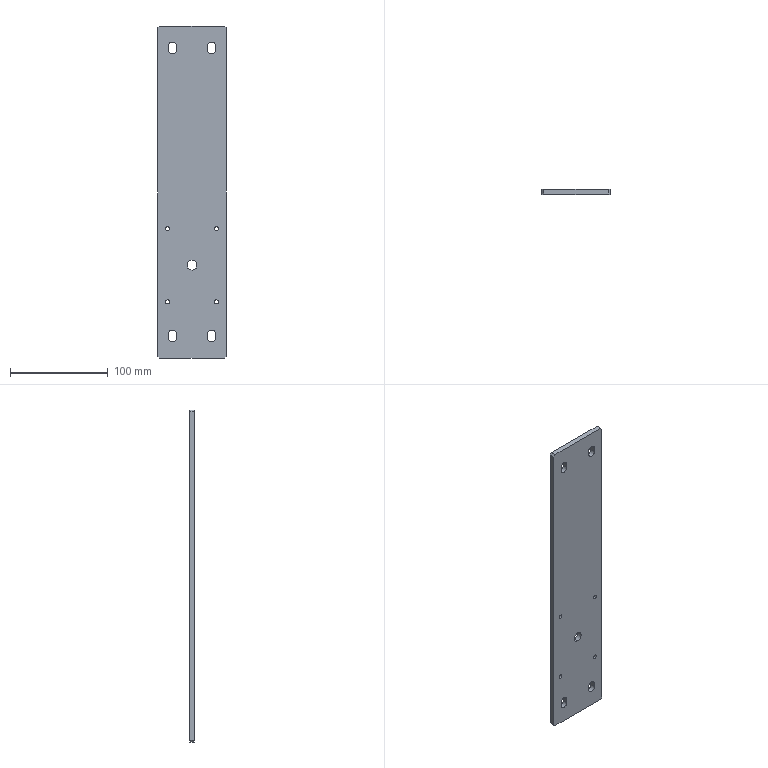Part | SolidWorks | features HoleWzd 2, Chamfer 1, Extrusion 1, ICE 1 | 1 solid | 40 faces | box 70 x 5 x 340 mm | volume 116578 mm3 | cylinder 22 | plane 18 | commonest cylinder face diameters 8.2 x12 4.2 x8 10 x2
STEP:
#1=CARTESIAN_POINT('',(-25.,0.,-110.4));
#2=VERTEX_POINT('',#1);
#3=CARTESIAN_POINT('',(-25.,0.,-114.6));
#4=VERTEX_POINT('',#3);
#5=CARTESIAN_POINT('',(-25.,0.,-112.5));
#6=DIRECTION('',(0.,-1.,0.));
#7=DIRECTION('',(0.,0.,-1.));
#8=AXIS2_PLACEMENT_3D('',#5,#6,#7);
#9=CIRCLE('',#8,2.1);
#10=EDGE_CURVE('',#2,#4,#9,.T.);
#11=ORIENTED_EDGE('',*,*,#10,.T.);
#12=CARTESIAN_POINT('',(-25.,5.,-114.6));
#13=VERTEX_POINT('',#12);
#14=CARTESIAN_POINT('',(-25.,5.,-114.6));
#15=DIRECTION('',(0.,1.,0.));
#16=VECTOR('',#15,1000.);
#17=LINE('',#14,#16);
#18=EDGE_CURVE('',#4,#13,#17,.T.);
#19=ORIENTED_EDGE('',*,*,#18,.T.);
#20=CARTESIAN_POINT('',(-25.,5.,-110.4));
#21=VERTEX_POINT('',#20);
#22=CARTESIAN_POINT('',(-25.,5.,-112.5));
#23=DIRECTION('',(0.,1.,0.));
#24=DIRECTION('',(0.,0.,1.));
#25=AXIS2_PLACEMENT_3D('',#22,#23,#24);
#26=CIRCLE('',#25,2.1);
#27=EDGE_CURVE('',#13,#21,#26,.T.);
#28=ORIENTED_EDGE('',*,*,#27,.T.);
#29=CARTESIAN_POINT('',(-25.,5.,-110.4));
#30=DIRECTION('',(0.,1.,0.));
#31=VECTOR('',#30,1000.);
#32=LINE('',#29,#31);
#33=EDGE_CURVE('',#2,#21,#32,.T.);
#34=ORIENTED_EDGE('',*,*,#33,.F.);
#35=EDGE_LOOP('',(#11,#19,#28,#34));
#36=FACE_OUTER_BOUND('',#35,.T.);
#37=CARTESIAN_POINT('',(-25.,5.,-112.5));
#38=DIRECTION('',(0.,1.,0.));
#39=DIRECTION('',(0.,0.,1.));
#40=AXIS2_PLACEMENT_3D('',#37,#38,#39);
#41=CYLINDRICAL_SURFACE('',#40,2.1);
#42=ADVANCED_FACE('',(#36),#41,.F.);
#43=CARTESIAN_POINT('',(25.,0.,-35.4));
#44=VERTEX_POINT('',#43);
#45=CARTESIAN_POINT('',(25.,0.,-39.6));
#46=VERTEX_POINT('',#45);
#47=CARTESIAN_POINT('',(25.,0.,-37.5));
#48=DIRECTION('',(0.,-1.,0.));
#49=DIRECTION('',(0.,0.,-1.));
#50=AXIS2_PLACEMENT_3D('',#47,#48,#49);
#51=CIRCLE('',#50,2.1);
#52=EDGE_CURVE('',#44,#46,#51,.T.);
#53=ORIENTED_EDGE('',*,*,#52,.T.);
#54=CARTESIAN_POINT('',(25.,5.,-39.6));
#55=VERTEX_POINT('',#54);
#56=CARTESIAN_POINT('',(25.,5.,-39.6));
#57=DIRECTION('',(0.,1.,0.));
#58=VECTOR('',#57,1000.);
#59=LINE('',#56,#58);
#60=EDGE_CURVE('',#46,#55,#59,.T.);
#61=ORIENTED_EDGE('',*,*,#60,.T.);
#62=CARTESIAN_POINT('',(25.,5.,-35.4));
#63=VERTEX_POINT('',#62);
#64=CARTESIAN_POINT('',(25.,5.,-37.5));
#65=DIRECTION('',(0.,1.,0.));
#66=DIRECTION('',(0.,0.,1.));
#67=AXIS2_PLACEMENT_3D('',#64,#65,#66);
#68=CIRCLE('',#67,2.1);
#69=EDGE_CURVE('',#55,#63,#68,.T.);
#70=ORIENTED_EDGE('',*,*,#69,.T.);
#71=CARTESIAN_POINT('',(25.,5.,-35.4));
#72=DIRECTION('',(0.,1.,0.));
#73=VECTOR('',#72,1000.);
#74=LINE('',#71,#73);
#75=EDGE_CURVE('',#44,#63,#74,.T.);
#76=ORIENTED_EDGE('',*,*,#75,.F.);
#77=EDGE_LOOP('',(#53,#61,#70,#76));
#78=FACE_OUTER_BOUND('',#77,.T.);
#79=CARTESIAN_POINT('',(25.,5.,-37.5));
#80=DIRECTION('',(0.,1.,0.));
#81=DIRECTION('',(0.,0.,1.));
#82=AXIS2_PLACEMENT_3D('',#79,#80,#81);
#83=CYLINDRICAL_SURFACE('',#82,2.1);
#84=ADVANCED_FACE('',(#78),#83,.F.);
#85=CARTESIAN_POINT('',(-25.,0.,-35.4));
#86=VERTEX_POINT('',#85);
#87=CARTESIAN_POINT('',(-25.,0.,-39.6));
#88=VERTEX_POINT('',#87);
#89=CARTESIAN_POINT('',(-25.,0.,-37.5));
#90=DIRECTION('',(0.,-1.,0.));
#91=DIRECTION('',(0.,0.,-1.));
#92=AXIS2_PLACEMENT_3D('',#89,#90,#91);
#93=CIRCLE('',#92,2.1);
#94=EDGE_CURVE('',#86,#88,#93,.T.);
#95=ORIENTED_EDGE('',*,*,#94,.T.);
#96=CARTESIAN_POINT('',(-25.,5.,-39.6));
#97=VERTEX_POINT('',#96);
#98=CARTESIAN_POINT('',(-25.,5.,-39.6));
#99=DIRECTION('',(0.,1.,0.));
#100=VECTOR('',#99,1000.);
#101=LINE('',#98,#100);
#102=EDGE_CURVE('',#88,#97,#101,.T.);
#103=ORIENTED_EDGE('',*,*,#102,.T.);
#104=CARTESIAN_POINT('',(-25.,5.,-35.4));
#105=VERTEX_POINT('',#104);
#106=CARTESIAN_POINT('',(-25.,5.,-37.5));
#107=DIRECTION('',(0.,1.,0.));
#108=DIRECTION('',(0.,0.,1.));
#109=AXIS2_PLACEMENT_3D('',#106,#107,#108);
#110=CIRCLE('',#109,2.1);
#111=EDGE_CURVE('',#97,#105,#110,.T.);
#112=ORIENTED_EDGE('',*,*,#111,.T.);
#113=CARTESIAN_POINT('',(-25.,5.,-35.4));
#114=DIRECTION('',(0.,1.,0.));
#115=VECTOR('',#114,1000.);
#116=LINE('',#113,#115);
#117=EDGE_CURVE('',#86,#105,#116,.T.);
#118=ORIENTED_EDGE('',*,*,#117,.F.);
#119=EDGE_LOOP('',(#95,#103,#112,#118));
#120=FACE_OUTER_BOUND('',#119,.T.);
#121=CARTESIAN_POINT('',(-25.,5.,-37.5));
#122=DIRECTION('',(0.,1.,0.));
#123=DIRECTION('',(0.,0.,1.));
#124=AXIS2_PLACEMENT_3D('',#121,#122,#123);
#125=CYLINDRICAL_SURFACE('',#124,2.1);
#126=ADVANCED_FACE('',(#120),#125,.F.);
#127=CARTESIAN_POINT('',(25.,0.,-110.4));
#128=VERTEX_POINT('',#127);
#129=CARTESIAN_POINT('',(25.,0.,-114.6));
#130=VERTEX_POINT('',#129);
#131=CARTESIAN_POINT('',(25.,0.,-112.5));
#132=DIRECTION('',(0.,-1.,0.));
#133=DIRECTION('',(0.,0.,-1.));
#134=AXIS2_PLACEMENT_3D('',#131,#132,#133);
#135=CIRCLE('',#134,2.1);
#136=EDGE_CURVE('',#128,#130,#135,.T.);
#137=ORIENTED_EDGE('',*,*,#136,.T.);
#138=CARTESIAN_POINT('',(25.,5.,-114.6));
#139=VERTEX_POINT('',#138);
#140=CARTESIAN_POINT('',(25.,5.,-114.6));
#141=DIRECTION('',(0.,1.,0.));
#142=VECTOR('',#141,1000.);
#143=LINE('',#140,#142);
#144=EDGE_CURVE('',#130,#139,#143,.T.);
#145=ORIENTED_EDGE('',*,*,#144,.T.);
#146=CARTESIAN_POINT('',(25.,5.,-110.4));
#147=VERTEX_POINT('',#146);
#148=CARTESIAN_POINT('',(25.,5.,-112.5));
#149=DIRECTION('',(0.,1.,0.));
#150=DIRECTION('',(0.,0.,1.));
#151=AXIS2_PLACEMENT_3D('',#148,#149,#150);
#152=CIRCLE('',#151,2.1);
#153=EDGE_CURVE('',#139,#147,#152,.T.);
#154=ORIENTED_EDGE('',*,*,#153,.T.);
#155=CARTESIAN_POINT('',(25.,5.,-110.4));
#156=DIRECTION('',(0.,1.,0.));
#157=VECTOR('',#156,1000.);
#158=LINE('',#155,#157);
#159=EDGE_CURVE('',#128,#147,#158,.T.);
#160=ORIENTED_EDGE('',*,*,#159,.F.);
#161=EDGE_LOOP('',(#137,#145,#154,#160));
#162=FACE_OUTER_BOUND('',#161,.T.);
#163=CARTESIAN_POINT('',(25.,5.,-112.5));
#164=DIRECTION('',(0.,1.,0.));
#165=DIRECTION('',(0.,0.,1.));
#166=AXIS2_PLACEMENT_3D('',#163,#164,#165);
#167=CYLINDRICAL_SURFACE('',#166,2.1);
#168=ADVANCED_FACE('',(#162),#167,.F.);
#169=CARTESIAN_POINT('',(0.,0.,-80.));
#170=VERTEX_POINT('',#169);
#171=CARTESIAN_POINT('',(0.,0.,-70.));
#172=VERTEX_POINT('',#171);
#173=CARTESIAN_POINT('',(0.,0.,-75.));
#174=DIRECTION('',(0.,1.,0.));
#175=DIRECTION('',(0.,0.,1.));
#176=AXIS2_PLACEMENT_3D('',#173,#174,#175);
#177=CIRCLE('',#176,5.);
#178=EDGE_CURVE('',#170,#172,#177,.T.);
#179=ORIENTED_EDGE('',*,*,#178,.F.);
#180=CARTESIAN_POINT('',(0.,5.,-80.));
#181=VERTEX_POINT('',#180);
#182=CARTESIAN_POINT('',(0.,0.,-80.));
#183=DIRECTION('',(0.,1.,0.));
#184=VECTOR('',#183,1000.);
#185=LINE('',#182,#184);
#186=EDGE_CURVE('',#170,#181,#185,.T.);
#187=ORIENTED_EDGE('',*,*,#186,.T.);
#188=CARTESIAN_POINT('',(0.,5.,-70.));
#189=VERTEX_POINT('',#188);
#190=CARTESIAN_POINT('',(0.,5.,-75.));
#191=DIRECTION('',(0.,1.,0.));
#192=DIRECTION('',(0.,0.,1.));
#193=AXIS2_PLACEMENT_3D('',#190,#191,#192);
#194=CIRCLE('',#193,5.);
#195=EDGE_CURVE('',#181,#189,#194,.T.);
#196=ORIENTED_EDGE('',*,*,#195,.T.);
#197=CARTESIAN_POINT('',(0.,0.,-70.));
#198=DIRECTION('',(0.,1.,0.));
#199=VECTOR('',#198,1000.);
#200=LINE('',#197,#199);
#201=EDGE_CURVE('',#172,#189,#200,.T.);
#202=ORIENTED_EDGE('',*,*,#201,.F.);
#203=EDGE_LOOP('',(#179,#187,#196,#202));
#204=FACE_OUTER_BOUND('',#203,.T.);
#205=CARTESIAN_POINT('',(0.,0.,-75.));
#206=DIRECTION('',(0.,1.,0.));
#207=DIRECTION('',(0.,0.,1.));
#208=AXIS2_PLACEMENT_3D('',#205,#206,#207);
#209=CYLINDRICAL_SURFACE('',#208,5.);
#210=ADVANCED_FACE('',(#204),#209,.F.);
#211=CARTESIAN_POINT('',(24.1,0.,-145.5));
#212=VERTEX_POINT('',#211);
#213=CARTESIAN_POINT('',(20.,0.,-141.4));
#214=VERTEX_POINT('',#213);
#215=CARTESIAN_POINT('',(20.,0.,-145.5));
#216=DIRECTION('',(0.,-1.,0.));
#217=DIRECTION('',(0.,0.,-1.));
#218=AXIS2_PLACEMENT_3D('',#215,#216,#217);
#219=CIRCLE('',#218,4.1);
#220=EDGE_CURVE('',#212,#214,#219,.T.);
#221=ORIENTED_EDGE('',*,*,#220,.T.);
#222=CARTESIAN_POINT('',(20.,5.,-141.4));
#223=VERTEX_POINT('',#222);
#224=CARTESIAN_POINT('',(20.,5.,-141.4));
#225=DIRECTION('',(0.,1.,0.));
#226=VECTOR('',#225,1000.);
#227=LINE('',#224,#226);
#228=EDGE_CURVE('',#214,#223,#227,.T.);
#229=ORIENTED_EDGE('',*,*,#228,.T.);
#230=CARTESIAN_POINT('',(24.1,5.,-145.5));
#231=VERTEX_POINT('',#230);
#232=CARTESIAN_POINT('',(20.,5.,-145.5));
#233=DIRECTION('',(0.,1.,0.));
#234=DIRECTION('',(0.,0.,1.));
#235=AXIS2_PLACEMENT_3D('',#232,#233,#234);
#236=CIRCLE('',#235,4.1);
#237=EDGE_CURVE('',#223,#231,#236,.T.);
#238=ORIENTED_EDGE('',*,*,#237,.T.);
#239=CARTESIAN_POINT('',(24.1,-10.,-145.5));
#240=DIRECTION('',(0.,-1.,0.));
#241=VECTOR('',#240,1000.);
#242=LINE('',#239,#241);
#243=EDGE_CURVE('',#231,#212,#242,.T.);
#244=ORIENTED_EDGE('',*,*,#243,.T.);
#245=EDGE_LOOP('',(#221,#229,#238,#244));
#246=FACE_OUTER_BOUND('',#245,.T.);
#247=CARTESIAN_POINT('',(20.,5.,-145.5));
#248=DIRECTION('',(0.,1.,0.));
#249=DIRECTION('',(0.,0.,1.));
#250=AXIS2_PLACEMENT_3D('',#247,#248,#249);
#251=CYLINDRICAL_SURFACE('',#250,4.1);
#252=ADVANCED_FACE('',(#246),#251,.F.);
#253=CARTESIAN_POINT('',(-15.9,0.,-145.5));
#254=VERTEX_POINT('',#253);
#255=CARTESIAN_POINT('',(-20.,0.,-141.4));
#256=VERTEX_POINT('',#255);
#257=CARTESIAN_POINT('',(-20.,0.,-145.5));
#258=DIRECTION('',(0.,-1.,0.));
#259=DIRECTION('',(0.,0.,-1.));
#260=AXIS2_PLACEMENT_3D('',#257,#258,#259);
#261=CIRCLE('',#260,4.1);
#262=EDGE_CURVE('',#254,#256,#261,.T.);
#263=ORIENTED_EDGE('',*,*,#262,.T.);
#264=CARTESIAN_POINT('',(-20.,5.,-141.4));
#265=VERTEX_POINT('',#264);
#266=CARTESIAN_POINT('',(-20.,5.,-141.4));
#267=DIRECTION('',(0.,1.,0.));
#268=VECTOR('',#267,1000.);
#269=LINE('',#266,#268);
#270=EDGE_CURVE('',#256,#265,#269,.T.);
#271=ORIENTED_EDGE('',*,*,#270,.T.);
#272=CARTESIAN_POINT('',(-15.9,5.,-145.5));
#273=VERTEX_POINT('',#272);
#274=CARTESIAN_POINT('',(-20.,5.,-145.5));
#275=DIRECTION('',(0.,1.,0.));
#276=DIRECTION('',(0.,0.,1.));
#277=AXIS2_PLACEMENT_3D('',#274,#275,#276);
#278=CIRCLE('',#277,4.1);
#279=EDGE_CURVE('',#265,#273,#278,.T.);
#280=ORIENTED_EDGE('',*,*,#279,.T.);
#281=CARTESIAN_POINT('',(-15.9,-10.,-145.5));
#282=DIRECTION('',(0.,-1.,0.));
#283=VECTOR('',#282,1000.);
#284=LINE('',#281,#283);
#285=EDGE_CURVE('',#273,#254,#284,.T.);
#286=ORIENTED_EDGE('',*,*,#285,.T.);
#287=EDGE_LOOP('',(#263,#271,#280,#286));
#288=FACE_OUTER_BOUND('',#287,.T.);
#289=CARTESIAN_POINT('',(-20.,5.,-145.5));
#290=DIRECTION('',(0.,1.,0.));
#291=DIRECTION('',(0.,0.,1.));
#292=AXIS2_PLACEMENT_3D('',#289,#290,#291);
#293=CYLINDRICAL_SURFACE('',#292,4.1);
#294=ADVANCED_FACE('',(#288),#293,.F.);
#295=CARTESIAN_POINT('',(-15.9,0.,149.5));
#296=VERTEX_POINT('',#295);
#297=CARTESIAN_POINT('',(-20.,0.,153.6));
#298=VERTEX_POINT('',#297);
#299=CARTESIAN_POINT('',(-20.,0.,149.5));
#300=DIRECTION('',(0.,-1.,0.));
#301=DIRECTION('',(0.,0.,-1.));
#302=AXIS2_PLACEMENT_3D('',#299,#300,#301);
#303=CIRCLE('',#302,4.1);
#304=EDGE_CURVE('',#296,#298,#303,.T.);
#305=ORIENTED_EDGE('',*,*,#304,.T.);
#306=CARTESIAN_POINT('',(-20.,5.,153.6));
#307=VERTEX_POINT('',#306);
#308=CARTESIAN_POINT('',(-20.,5.,153.6));
#309=DIRECTION('',(0.,1.,0.));
#310=VECTOR('',#309,1000.);
#311=LINE('',#308,#310);
#312=EDGE_CURVE('',#298,#307,#311,.T.);
#313=ORIENTED_EDGE('',*,*,#312,.T.);
#314=CARTESIAN_POINT('',(-15.9,5.,149.5));
#315=VERTEX_POINT('',#314);
#316=CARTESIAN_POINT('',(-20.,5.,149.5));
#317=DIRECTION('',(0.,1.,0.));
#318=DIRECTION('',(0.,0.,1.));
#319=AXIS2_PLACEMENT_3D('',#316,#317,#318);
#320=CIRCLE('',#319,4.1);
#321=EDGE_CURVE('',#307,#315,#320,.T.);
#322=ORIENTED_EDGE('',*,*,#321,.T.);
#323=CARTESIAN_POINT('',(-15.9,-10.,149.5));
#324=DIRECTION('',(0.,-1.,0.));
#325=VECTOR('',#324,1000.);
#326=LINE('',#323,#325);
#327=EDGE_CURVE('',#315,#296,#326,.T.);
#328=ORIENTED_EDGE('',*,*,#327,.T.);
#329=EDGE_LOOP('',(#305,#313,#322,#328));
#330=FACE_OUTER_BOUND('',#329,.T.);
#331=CARTESIAN_POINT('',(-20.,5.,149.5));
#332=DIRECTION('',(0.,1.,0.));
#333=DIRECTION('',(0.,0.,1.));
#334=AXIS2_PLACEMENT_3D('',#331,#332,#333);
#335=CYLINDRICAL_SURFACE('',#334,4.1);
#336=ADVANCED_FACE('',(#330),#335,.F.);
#337=CARTESIAN_POINT('',(24.1,0.,149.5));
#338=VERTEX_POINT('',#337);
#339=CARTESIAN_POINT('',(20.,0.,153.6));
#340=VERTEX_POINT('',#339);
#341=CARTESIAN_POINT('',(20.,0.,149.5));
#342=DIRECTION('',(0.,-1.,0.));
#343=DIRECTION('',(0.,0.,-1.));
#344=AXIS2_PLACEMENT_3D('',#341,#342,#343);
#345=CIRCLE('',#344,4.1);
#346=EDGE_CURVE('',#338,#340,#345,.T.);
#347=ORIENTED_EDGE('',*,*,#346,.T.);
#348=CARTESIAN_POINT('',(20.,5.,153.6));
#349=VERTEX_POINT('',#348);
#350=CARTESIAN_POINT('',(20.,5.,153.6));
#351=DIRECTION('',(0.,1.,0.));
#352=VECTOR('',#351,1000.);
#353=LINE('',#350,#352);
#354=EDGE_CURVE('',#340,#349,#353,.T.);
#355=ORIENTED_EDGE('',*,*,#354,.T.);
#356=CARTESIAN_POINT('',(24.1,5.,149.5));
#357=VERTEX_POINT('',#356);
#358=CARTESIAN_POINT('',(20.,5.,149.5));
#359=DIRECTION('',(0.,1.,0.));
#360=DIRECTION('',(0.,0.,1.));
#361=AXIS2_PLACEMENT_3D('',#358,#359,#360);
#362=CIRCLE('',#361,4.1);
#363=EDGE_CURVE('',#349,#357,#362,.T.);
#364=ORIENTED_EDGE('',*,*,#363,.T.);
#365=CARTESIAN_POINT('',(24.1,-10.,149.5));
#366=DIRECTION('',(0.,-1.,0.));
#367=VECTOR('',#366,1000.);
#368=LINE('',#365,#367);
#369=EDGE_CURVE('',#357,#338,#368,.T.);
#370=ORIENTED_EDGE('',*,*,#369,.T.);
#371=EDGE_LOOP('',(#347,#355,#364,#370));
#372=FACE_OUTER_BOUND('',#371,.T.);
#373=CARTESIAN_POINT('',(20.,5.,149.5));
#374=DIRECTION('',(0.,1.,0.));
#375=DIRECTION('',(0.,0.,1.));
#376=AXIS2_PLACEMENT_3D('',#373,#374,#375);
#377=CYLINDRICAL_SURFACE('',#376,4.1);
#378=ADVANCED_FACE('',(#372),#377,.F.);
#379=CARTESIAN_POINT('',(35.,0.,168.));
#380=VERTEX_POINT('',#379);
#381=CARTESIAN_POINT('',(35.,0.,-168.));
#382=VERTEX_POINT('',#381);
#383=CARTESIAN_POINT('',(35.,0.,170.));
#384=DIRECTION('',(0.,0.,-1.));
#385=VECTOR('',#384,1000.);
#386=LINE('',#383,#385);
#387=EDGE_CURVE('',#380,#382,#386,.T.);
#388=ORIENTED_EDGE('',*,*,#387,.T.);
#389=CARTESIAN_POINT('',(35.,5.,-168.));
#390=VERTEX_POINT('',#389);
#391=CARTESIAN_POINT('',(35.,5.,-168.));
#392=DIRECTION('',(0.,1.,0.));
#393=VECTOR('',#392,1000.);
#394=LINE('',#391,#393);
#395=EDGE_CURVE('',#382,#390,#394,.T.);
#396=ORIENTED_EDGE('',*,*,#395,.T.);
#397=CARTESIAN_POINT('',(35.,5.,168.));
#398=VERTEX_POINT('',#397);
#399=CARTESIAN_POINT('',(35.,5.,170.));
#400=DIRECTION('',(0.,0.,-1.));
#401=VECTOR('',#400,1000.);
#402=LINE('',#399,#401);
#403=EDGE_CURVE('',#398,#390,#402,.T.);
#404=ORIENTED_EDGE('',*,*,#403,.F.);
#405=CARTESIAN_POINT('',(35.,5.,168.));
#406=DIRECTION('',(0.,-1.,0.));
#407=VECTOR('',#406,1000.);
#408=LINE('',#405,#407);
#409=EDGE_CURVE('',#398,#380,#408,.T.);
#410=ORIENTED_EDGE('',*,*,#409,.T.);
#411=EDGE_LOOP('',(#388,#396,#404,#410));
#412=FACE_OUTER_BOUND('',#411,.T.);
#413=CARTESIAN_POINT('',(35.,5.,170.));
#414=DIRECTION('',(-1.,0.,0.));
#415=DIRECTION('',(0.,0.,1.));
#416=AXIS2_PLACEMENT_3D('',#413,#414,#415);
#417=PLANE('',#416);
#418=ADVANCED_FACE('',(#412),#417,.F.);
#419=CARTESIAN_POINT('',(33.,0.,-170.));
#420=VERTEX_POINT('',#419);
#421=CARTESIAN_POINT('',(-33.,0.,-170.));
#422=VERTEX_POINT('',#421);
#423=CARTESIAN_POINT('',(-35.,0.,-170.));
#424=DIRECTION('',(-1.,0.,0.));
#425=VECTOR('',#424,1000.);
#426=LINE('',#423,#425);
#427=EDGE_CURVE('',#420,#422,#426,.T.);
#428=ORIENTED_EDGE('',*,*,#427,.T.);
#429=CARTESIAN_POINT('',(-33.,5.,-170.));
#430=VERTEX_POINT('',#429);
#431=CARTESIAN_POINT('',(-33.,5.,-170.));
#432=DIRECTION('',(0.,1.,0.));
#433=VECTOR('',#432,1000.);
#434=LINE('',#431,#433);
#435=EDGE_CURVE('',#422,#430,#434,.T.);
#436=ORIENTED_EDGE('',*,*,#435,.T.);
#437=CARTESIAN_POINT('',(33.,5.,-170.));
#438=VERTEX_POINT('',#437);
#439=CARTESIAN_POINT('',(-35.,5.,-170.));
#440=DIRECTION('',(-1.,0.,0.));
#441=VECTOR('',#440,1000.);
#442=LINE('',#439,#441);
#443=EDGE_CURVE('',#438,#430,#442,.T.);
#444=ORIENTED_EDGE('',*,*,#443,.F.);
#445=CARTESIAN_POINT('',(33.,5.,-170.));
#446=DIRECTION('',(0.,-1.,0.));
#447=VECTOR('',#446,1000.);
#448=LINE('',#445,#447);
#449=EDGE_CURVE('',#438,#420,#448,.T.);
#450=ORIENTED_EDGE('',*,*,#449,.T.);
#451=EDGE_LOOP('',(#428,#436,#444,#450));
#452=FACE_OUTER_BOUND('',#451,.T.);
#453=CARTESIAN_POINT('',(-35.,5.,-170.));
#454=DIRECTION('',(0.,0.,1.));
#455=DIRECTION('',(1.,0.,0.));
#456=AXIS2_PLACEMENT_3D('',#453,#454,#455);
#457=PLANE('',#456);
#458=ADVANCED_FACE('',(#452),#457,.F.);
#459=CARTESIAN_POINT('',(-35.,5.,-168.));
#460=VERTEX_POINT('',#459);
#461=CARTESIAN_POINT('',(-35.,5.,168.));
#462=VERTEX_POINT('',#461);
#463=CARTESIAN_POINT('',(-35.,5.,170.));
#464=DIRECTION('',(0.,0.,1.));
#465=VECTOR('',#464,1000.);
#466=LINE('',#463,#465);
#467=EDGE_CURVE('',#460,#462,#466,.T.);
#468=ORIENTED_EDGE('',*,*,#467,.F.);
#469=CARTESIAN_POINT('',(-35.,0.,-168.));
#470=VERTEX_POINT('',#469);
#471=CARTESIAN_POINT('',(-35.,5.,-168.));
#472=DIRECTION('',(0.,-1.,0.));
#473=VECTOR('',#472,1000.);
#474=LINE('',#471,#473);
#475=EDGE_CURVE('',#460,#470,#474,.T.);
#476=ORIENTED_EDGE('',*,*,#475,.T.);
#477=CARTESIAN_POINT('',(-35.,0.,168.));
#478=VERTEX_POINT('',#477);
#479=CARTESIAN_POINT('',(-35.,0.,170.));
#480=DIRECTION('',(0.,0.,1.));
#481=VECTOR('',#480,1000.);
#482=LINE('',#479,#481);
#483=EDGE_CURVE('',#470,#478,#482,.T.);
#484=ORIENTED_EDGE('',*,*,#483,.T.);
#485=CARTESIAN_POINT('',(-35.,5.,168.));
#486=DIRECTION('',(0.,1.,0.));
#487=VECTOR('',#486,1000.);
#488=LINE('',#485,#487);
#489=EDGE_CURVE('',#478,#462,#488,.T.);
#490=ORIENTED_EDGE('',*,*,#489,.T.);
#491=EDGE_LOOP('',(#468,#476,#484,#490));
#492=FACE_OUTER_BOUND('',#491,.T.);
#493=CARTESIAN_POINT('',(-35.,5.,170.));
#494=DIRECTION('',(1.,0.,0.));
#495=DIRECTION('',(0.,0.,-1.));
#496=AXIS2_PLACEMENT_3D('',#493,#494,#495);
#497=PLANE('',#496);
#498=ADVANCED_FACE('',(#492),#497,.F.);
#499=CARTESIAN_POINT('',(-33.,0.,170.));
#500=VERTEX_POINT('',#499);
#501=CARTESIAN_POINT('',(33.,0.,170.));
#502=VERTEX_POINT('',#501);
#503=CARTESIAN_POINT('',(-35.,0.,170.));
#504=DIRECTION('',(1.,0.,0.));
#505=VECTOR('',#504,1000.);
#506=LINE('',#503,#505);
#507=EDGE_CURVE('',#500,#502,#506,.T.);
#508=ORIENTED_EDGE('',*,*,#507,.T.);
#509=CARTESIAN_POINT('',(33.,5.,170.));
#510=VERTEX_POINT('',#509);
#511=CARTESIAN_POINT('',(33.,5.,170.));
#512=DIRECTION('',(0.,1.,0.));
#513=VECTOR('',#512,1000.);
#514=LINE('',#511,#513);
#515=EDGE_CURVE('',#502,#510,#514,.T.);
#516=ORIENTED_EDGE('',*,*,#515,.T.);
#517=CARTESIAN_POINT('',(-33.,5.,170.));
#518=VERTEX_POINT('',#517);
#519=CARTESIAN_POINT('',(-35.,5.,170.));
#520=DIRECTION('',(1.,0.,0.));
#521=VECTOR('',#520,1000.);
#522=LINE('',#519,#521);
#523=EDGE_CURVE('',#518,#510,#522,.T.);
#524=ORIENTED_EDGE('',*,*,#523,.F.);
#525=CARTESIAN_POINT('',(-33.,5.,170.));
#526=DIRECTION('',(0.,-1.,0.));
#527=VECTOR('',#526,1000.);
#528=LINE('',#525,#527);
#529=EDGE_CURVE('',#518,#500,#528,.T.);
#530=ORIENTED_EDGE('',*,*,#529,.T.);
#531=EDGE_LOOP('',(#508,#516,#524,#530));
#532=FACE_OUTER_BOUND('',#531,.T.);
#533=CARTESIAN_POINT('',(-35.,5.,170.));
#534=DIRECTION('',(0.,0.,-1.));
#535=DIRECTION('',(-1.,0.,0.));
#536=AXIS2_PLACEMENT_3D('',#533,#534,#535);
#537=PLANE('',#536);
#538=ADVANCED_FACE('',(#532),#537,.F.);
#539=CARTESIAN_POINT('',(-25.,5.,-112.5));
#540=DIRECTION('',(0.,1.,0.));
#541=DIRECTION('',(0.,0.,1.));
#542=AXIS2_PLACEMENT_3D('',#539,#540,#541);
#543=CIRCLE('',#542,2.1);
#544=EDGE_CURVE('',#21,#13,#543,.T.);
#545=ORIENTED_EDGE('',*,*,#544,.F.);
#546=ORIENTED_EDGE('',*,*,#27,.F.);
#547=EDGE_LOOP('',(#545,#546));
#548=FACE_BOUND('',#547,.T.);
#549=CARTESIAN_POINT('',(25.,5.,-37.5));
#550=DIRECTION('',(0.,1.,0.));
#551=DIRECTION('',(0.,0.,1.));
#552=AXIS2_PLACEMENT_3D('',#549,#550,#551);
#553=CIRCLE('',#552,2.1);
#554=EDGE_CURVE('',#63,#55,#553,.T.);
#555=ORIENTED_EDGE('',*,*,#554,.F.);
#556=ORIENTED_EDGE('',*,*,#69,.F.);
#557=EDGE_LOOP('',(#555,#556));
#558=FACE_BOUND('',#557,.T.);
#559=CARTESIAN_POINT('',(-25.,5.,-37.5));
#560=DIRECTION('',(0.,1.,0.));
#561=DIRECTION('',(0.,0.,1.));
#562=AXIS2_PLACEMENT_3D('',#559,#560,#561);
#563=CIRCLE('',#562,2.1);
#564=EDGE_CURVE('',#105,#97,#563,.T.);
#565=ORIENTED_EDGE('',*,*,#564,.F.);
#566=ORIENTED_EDGE('',*,*,#111,.F.);
#567=EDGE_LOOP('',(#565,#566));
#568=FACE_BOUND('',#567,.T.);
#569=CARTESIAN_POINT('',(25.,5.,-112.5));
#570=DIRECTION('',(0.,1.,0.));
#571=DIRECTION('',(0.,0.,1.));
#572=AXIS2_PLACEMENT_3D('',#569,#570,#571);
#573=CIRCLE('',#572,2.1);
#574=EDGE_CURVE('',#147,#139,#573,.T.);
#575=ORIENTED_EDGE('',*,*,#574,.F.);
#576=ORIENTED_EDGE('',*,*,#153,.F.);
#577=EDGE_LOOP('',(#575,#576));
#578=FACE_BOUND('',#577,.T.);
#579=CARTESIAN_POINT('',(0.,5.,-75.));
#580=DIRECTION('',(0.,1.,0.));
#581=DIRECTION('',(0.,0.,1.));
#582=AXIS2_PLACEMENT_3D('',#579,#580,#581);
#583=CIRCLE('',#582,5.);
#584=EDGE_CURVE('',#189,#181,#583,.T.);
#585=ORIENTED_EDGE('',*,*,#584,.F.);
#586=ORIENTED_EDGE('',*,*,#195,.F.);
#587=EDGE_LOOP('',(#585,#586));
#588=FACE_BOUND('',#587,.T.);
#589=CARTESIAN_POINT('',(15.9,5.,-145.5));
#590=VERTEX_POINT('',#589);
#591=CARTESIAN_POINT('',(15.9,5.,-149.5));
#592=VERTEX_POINT('',#591);
#593=CARTESIAN_POINT('',(15.9,5.,-145.5));
#594=DIRECTION('',(0.,0.,-1.));
#595=VECTOR('',#594,1000.);
#596=LINE('',#593,#595);
#597=EDGE_CURVE('',#590,#592,#596,.T.);
#598=ORIENTED_EDGE('',*,*,#597,.T.);
#599=CARTESIAN_POINT('',(24.1,5.,-149.5));
#600=VERTEX_POINT('',#599);
#601=CARTESIAN_POINT('',(20.,5.,-149.5));
#602=DIRECTION('',(0.,1.,0.));
#603=DIRECTION('',(0.,0.,1.));
#604=AXIS2_PLACEMENT_3D('',#601,#602,#603);
#605=CIRCLE('',#604,4.1);
#606=EDGE_CURVE('',#600,#592,#605,.T.);
#607=ORIENTED_EDGE('',*,*,#606,.F.);
#608=CARTESIAN_POINT('',(24.1,5.,-145.5));
#609=DIRECTION('',(0.,0.,-1.));
#610=VECTOR('',#609,1000.);
#611=LINE('',#608,#610);
#612=EDGE_CURVE('',#231,#600,#611,.T.);
#613=ORIENTED_EDGE('',*,*,#612,.F.);
#614=ORIENTED_EDGE('',*,*,#237,.F.);
#615=CARTESIAN_POINT('',(20.,5.,-145.5));
#616=DIRECTION('',(0.,1.,0.));
#617=DIRECTION('',(0.,0.,1.));
#618=AXIS2_PLACEMENT_3D('',#615,#616,#617);
#619=CIRCLE('',#618,4.1);
#620=EDGE_CURVE('',#590,#223,#619,.T.);
#621=ORIENTED_EDGE('',*,*,#620,.F.);
#622=EDGE_LOOP('',(#598,#607,#613,#614,#621));
#623=FACE_BOUND('',#622,.T.);
#624=CARTESIAN_POINT('',(-24.1,5.,-145.5));
#625=VERTEX_POINT('',#624);
#626=CARTESIAN_POINT('',(-24.1,5.,-149.5));
#627=VERTEX_POINT('',#626);
#628=CARTESIAN_POINT('',(-24.1,5.,-145.5));
#629=DIRECTION('',(0.,0.,-1.));
#630=VECTOR('',#629,1000.);
#631=LINE('',#628,#630);
#632=EDGE_CURVE('',#625,#627,#631,.T.);
#633=ORIENTED_EDGE('',*,*,#632,.T.);
#634=CARTESIAN_POINT('',(-15.9,5.,-149.5));
#635=VERTEX_POINT('',#634);
#636=CARTESIAN_POINT('',(-20.,5.,-149.5));
#637=DIRECTION('',(0.,1.,0.));
#638=DIRECTION('',(0.,0.,1.));
#639=AXIS2_PLACEMENT_3D('',#636,#637,#638);
#640=CIRCLE('',#639,4.1);
#641=EDGE_CURVE('',#635,#627,#640,.T.);
#642=ORIENTED_EDGE('',*,*,#641,.F.);
#643=CARTESIAN_POINT('',(-15.9,5.,-145.5));
#644=DIRECTION('',(0.,0.,-1.));
#645=VECTOR('',#644,1000.);
#646=LINE('',#643,#645);
#647=EDGE_CURVE('',#273,#635,#646,.T.);
#648=ORIENTED_EDGE('',*,*,#647,.F.);
#649=ORIENTED_EDGE('',*,*,#279,.F.);
#650=CARTESIAN_POINT('',(-20.,5.,-145.5));
#651=DIRECTION('',(0.,1.,0.));
#652=DIRECTION('',(0.,0.,1.));
#653=AXIS2_PLACEMENT_3D('',#650,#651,#652);
#654=CIRCLE('',#653,4.1);
#655=EDGE_CURVE('',#625,#265,#654,.T.);
#656=ORIENTED_EDGE('',*,*,#655,.F.);
#657=EDGE_LOOP('',(#633,#642,#648,#649,#656));
#658=FACE_BOUND('',#657,.T.);
#659=CARTESIAN_POINT('',(-15.9,5.,145.5));
#660=VERTEX_POINT('',#659);
#661=CARTESIAN_POINT('',(-15.9,5.,149.5));
#662=DIRECTION('',(0.,0.,-1.));
#663=VECTOR('',#662,1000.);
#664=LINE('',#661,#663);
#665=EDGE_CURVE('',#315,#660,#664,.T.);
#666=ORIENTED_EDGE('',*,*,#665,.F.);
#667=ORIENTED_EDGE('',*,*,#321,.F.);
#668=CARTESIAN_POINT('',(-24.1,5.,149.5));
#669=VERTEX_POINT('',#668);
#670=CARTESIAN_POINT('',(-20.,5.,149.5));
#671=DIRECTION('',(0.,1.,0.));
#672=DIRECTION('',(0.,0.,1.));
#673=AXIS2_PLACEMENT_3D('',#670,#671,#672);
#674=CIRCLE('',#673,4.1);
#675=EDGE_CURVE('',#669,#307,#674,.T.);
#676=ORIENTED_EDGE('',*,*,#675,.F.);
#677=CARTESIAN_POINT('',(-24.1,5.,145.5));
#678=VERTEX_POINT('',#677);
#679=CARTESIAN_POINT('',(-24.1,5.,149.5));
#680=DIRECTION('',(0.,0.,-1.));
#681=VECTOR('',#680,1000.);
#682=LINE('',#679,#681);
#683=EDGE_CURVE('',#669,#678,#682,.T.);
#684=ORIENTED_EDGE('',*,*,#683,.T.);
#685=CARTESIAN_POINT('',(-20.,5.,145.5));
#686=DIRECTION('',(0.,1.,0.));
#687=DIRECTION('',(0.,0.,1.));
#688=AXIS2_PLACEMENT_3D('',#685,#686,#687);
#689=CIRCLE('',#688,4.1);
#690=EDGE_CURVE('',#660,#678,#689,.T.);
#691=ORIENTED_EDGE('',*,*,#690,.F.);
#692=EDGE_LOOP('',(#666,#667,#676,#684,#691));
#693=FACE_BOUND('',#692,.T.);
#694=CARTESIAN_POINT('',(15.9,5.,149.5));
#695=VERTEX_POINT('',#694);
#696=CARTESIAN_POINT('',(20.,5.,149.5));
#697=DIRECTION('',(0.,1.,0.));
#698=DIRECTION('',(0.,0.,1.));
#699=AXIS2_PLACEMENT_3D('',#696,#697,#698);
#700=CIRCLE('',#699,4.1);
#701=EDGE_CURVE('',#695,#349,#700,.T.);
#702=ORIENTED_EDGE('',*,*,#701,.F.);
#703=CARTESIAN_POINT('',(15.9,5.,145.5));
#704=VERTEX_POINT('',#703);
#705=CARTESIAN_POINT('',(15.9,5.,149.5));
#706=DIRECTION('',(0.,0.,-1.));
#707=VECTOR('',#706,1000.);
#708=LINE('',#705,#707);
#709=EDGE_CURVE('',#695,#704,#708,.T.);
#710=ORIENTED_EDGE('',*,*,#709,.T.);
#711=CARTESIAN_POINT('',(24.1,5.,145.5));
#712=VERTEX_POINT('',#711);
#713=CARTESIAN_POINT('',(20.,5.,145.5));
#714=DIRECTION('',(0.,1.,0.));
#715=DIRECTION('',(0.,0.,1.));
#716=AXIS2_PLACEMENT_3D('',#713,#714,#715);
#717=CIRCLE('',#716,4.1);
#718=EDGE_CURVE('',#712,#704,#717,.T.);
#719=ORIENTED_EDGE('',*,*,#718,.F.);
#720=CARTESIAN_POINT('',(24.1,5.,149.5));
#721=DIRECTION('',(0.,0.,-1.));
#722=VECTOR('',#721,1000.);
#723=LINE('',#720,#722);
#724=EDGE_CURVE('',#357,#712,#723,.T.);
#725=ORIENTED_EDGE('',*,*,#724,.F.);
#726=ORIENTED_EDGE('',*,*,#363,.F.);
#727=EDGE_LOOP('',(#702,#710,#719,#725,#726));
#728=FACE_BOUND('',#727,.T.);
#729=ORIENTED_EDGE('',*,*,#443,.T.);
#730=CARTESIAN_POINT('',(-35.,5.,-168.));
#731=DIRECTION('',(-0.7071,0.,0.7071));
#732=VECTOR('',#731,1000.);
#733=LINE('',#730,#732);
#734=EDGE_CURVE('',#430,#460,#733,.T.);
#735=ORIENTED_EDGE('',*,*,#734,.T.);
#736=ORIENTED_EDGE('',*,*,#467,.T.);
#737=CARTESIAN_POINT('',(-33.,5.,170.));
#738=DIRECTION('',(0.7071,0.,0.7071));
#739=VECTOR('',#738,1000.);
#740=LINE('',#737,#739);
#741=EDGE_CURVE('',#462,#518,#740,.T.);
#742=ORIENTED_EDGE('',*,*,#741,.T.);
#743=ORIENTED_EDGE('',*,*,#523,.T.);
#744=CARTESIAN_POINT('',(35.,5.,168.));
#745=DIRECTION('',(0.7071,0.,-0.7071));
#746=VECTOR('',#745,1000.);
#747=LINE('',#744,#746);
#748=EDGE_CURVE('',#510,#398,#747,.T.);
#749=ORIENTED_EDGE('',*,*,#748,.T.);
#750=ORIENTED_EDGE('',*,*,#403,.T.);
#751=CARTESIAN_POINT('',(33.,5.,-170.));
#752=DIRECTION('',(-0.7071,0.,-0.7071));
#753=VECTOR('',#752,1000.);
#754=LINE('',#751,#753);
#755=EDGE_CURVE('',#390,#438,#754,.T.);
#756=ORIENTED_EDGE('',*,*,#755,.T.);
#757=EDGE_LOOP('',(#729,#735,#736,#742,#743,#749,#750,#756));
#758=FACE_OUTER_BOUND('',#757,.T.);
#759=CARTESIAN_POINT('',(0.,5.,0.));
#760=DIRECTION('',(0.,-1.,0.));
#761=DIRECTION('',(0.,0.,-1.));
#762=AXIS2_PLACEMENT_3D('',#759,#760,#761);
#763=PLANE('',#762);
#764=ADVANCED_FACE('',(#548,#558,#568,#578,#588,#623,#658,#693,#728,#758),#763,.F.);
#765=ORIENTED_EDGE('',*,*,#10,.F.);
#766=CARTESIAN_POINT('',(-25.,0.,-112.5));
#767=DIRECTION('',(0.,-1.,0.));
#768=DIRECTION('',(0.,0.,-1.));
#769=AXIS2_PLACEMENT_3D('',#766,#767,#768);
#770=CIRCLE('',#769,2.1);
#771=EDGE_CURVE('',#4,#2,#770,.T.);
#772=ORIENTED_EDGE('',*,*,#771,.F.);
#773=EDGE_LOOP('',(#765,#772));
#774=FACE_BOUND('',#773,.T.);
#775=ORIENTED_EDGE('',*,*,#52,.F.);
#776=CARTESIAN_POINT('',(25.,0.,-37.5));
#777=DIRECTION('',(0.,-1.,0.));
#778=DIRECTION('',(0.,0.,-1.));
#779=AXIS2_PLACEMENT_3D('',#776,#777,#778);
#780=CIRCLE('',#779,2.1);
#781=EDGE_CURVE('',#46,#44,#780,.T.);
#782=ORIENTED_EDGE('',*,*,#781,.F.);
#783=EDGE_LOOP('',(#775,#782));
#784=FACE_BOUND('',#783,.T.);
#785=ORIENTED_EDGE('',*,*,#94,.F.);
#786=CARTESIAN_POINT('',(-25.,0.,-37.5));
#787=DIRECTION('',(0.,-1.,0.));
#788=DIRECTION('',(0.,0.,-1.));
#789=AXIS2_PLACEMENT_3D('',#786,#787,#788);
#790=CIRCLE('',#789,2.1);
#791=EDGE_CURVE('',#88,#86,#790,.T.);
#792=ORIENTED_EDGE('',*,*,#791,.F.);
#793=EDGE_LOOP('',(#785,#792));
#794=FACE_BOUND('',#793,.T.);
#795=ORIENTED_EDGE('',*,*,#136,.F.);
#796=CARTESIAN_POINT('',(25.,0.,-112.5));
#797=DIRECTION('',(0.,-1.,0.));
#798=DIRECTION('',(0.,0.,-1.));
#799=AXIS2_PLACEMENT_3D('',#796,#797,#798);
#800=CIRCLE('',#799,2.1);
#801=EDGE_CURVE('',#130,#128,#800,.T.);
#802=ORIENTED_EDGE('',*,*,#801,.F.);
#803=EDGE_LOOP('',(#795,#802));
#804=FACE_BOUND('',#803,.T.);
#805=CARTESIAN_POINT('',(0.,0.,-75.));
#806=DIRECTION('',(0.,1.,0.));
#807=DIRECTION('',(0.,0.,1.));
#808=AXIS2_PLACEMENT_3D('',#805,#806,#807);
#809=CIRCLE('',#808,5.);
#810=EDGE_CURVE('',#172,#170,#809,.T.);
#811=ORIENTED_EDGE('',*,*,#810,.T.);
#812=ORIENTED_EDGE('',*,*,#178,.T.);
#813=EDGE_LOOP('',(#811,#812));
#814=FACE_BOUND('',#813,.T.);
#815=CARTESIAN_POINT('',(15.9,0.,-145.5));
#816=VERTEX_POINT('',#815);
#817=CARTESIAN_POINT('',(15.9,0.,-149.5));
#818=VERTEX_POINT('',#817);
#819=CARTESIAN_POINT('',(15.9,0.,0.));
#820=DIRECTION('',(0.,0.,-1.));
#821=VECTOR('',#820,1000.);
#822=LINE('',#819,#821);
#823=EDGE_CURVE('',#816,#818,#822,.T.);
#824=ORIENTED_EDGE('',*,*,#823,.F.);
#825=CARTESIAN_POINT('',(20.,0.,-145.5));
#826=DIRECTION('',(0.,-1.,0.));
#827=DIRECTION('',(0.,0.,-1.));
#828=AXIS2_PLACEMENT_3D('',#825,#826,#827);
#829=CIRCLE('',#828,4.1);
#830=EDGE_CURVE('',#214,#816,#829,.T.);
#831=ORIENTED_EDGE('',*,*,#830,.F.);
#832=ORIENTED_EDGE('',*,*,#220,.F.);
#833=CARTESIAN_POINT('',(24.1,0.,-149.5));
#834=VERTEX_POINT('',#833);
#835=CARTESIAN_POINT('',(24.1,0.,0.));
#836=DIRECTION('',(0.,0.,1.));
#837=VECTOR('',#836,1000.);
#838=LINE('',#835,#837);
#839=EDGE_CURVE('',#834,#212,#838,.T.);
#840=ORIENTED_EDGE('',*,*,#839,.F.);
#841=CARTESIAN_POINT('',(20.,0.,-149.5));
#842=DIRECTION('',(0.,-1.,0.));
#843=DIRECTION('',(0.,0.,-1.));
#844=AXIS2_PLACEMENT_3D('',#841,#842,#843);
#845=CIRCLE('',#844,4.1);
#846=EDGE_CURVE('',#818,#834,#845,.T.);
#847=ORIENTED_EDGE('',*,*,#846,.F.);
#848=EDGE_LOOP('',(#824,#831,#832,#840,#847));
#849=FACE_BOUND('',#848,.T.);
#850=CARTESIAN_POINT('',(-24.1,0.,-149.5));
#851=VERTEX_POINT('',#850);
#852=CARTESIAN_POINT('',(-15.9,0.,-149.5));
#853=VERTEX_POINT('',#852);
#854=CARTESIAN_POINT('',(-20.,0.,-149.5));
#855=DIRECTION('',(0.,-1.,0.));
#856=DIRECTION('',(0.,0.,-1.));
#857=AXIS2_PLACEMENT_3D('',#854,#855,#856);
#858=CIRCLE('',#857,4.1);
#859=EDGE_CURVE('',#851,#853,#858,.T.);
#860=ORIENTED_EDGE('',*,*,#859,.F.);
#861=CARTESIAN_POINT('',(-24.1,0.,-145.5));
#862=VERTEX_POINT('',#861);
#863=CARTESIAN_POINT('',(-24.1,0.,0.));
#864=DIRECTION('',(0.,0.,-1.));
#865=VECTOR('',#864,1000.);
#866=LINE('',#863,#865);
#867=EDGE_CURVE('',#862,#851,#866,.T.);
#868=ORIENTED_EDGE('',*,*,#867,.F.);
#869=CARTESIAN_POINT('',(-20.,0.,-145.5));
#870=DIRECTION('',(0.,-1.,0.));
#871=DIRECTION('',(0.,0.,-1.));
#872=AXIS2_PLACEMENT_3D('',#869,#870,#871);
#873=CIRCLE('',#872,4.1);
#874=EDGE_CURVE('',#256,#862,#873,.T.);
#875=ORIENTED_EDGE('',*,*,#874,.F.);
#876=ORIENTED_EDGE('',*,*,#262,.F.);
#877=CARTESIAN_POINT('',(-15.9,0.,0.));
#878=DIRECTION('',(0.,0.,1.));
#879=VECTOR('',#878,1000.);
#880=LINE('',#877,#879);
#881=EDGE_CURVE('',#853,#254,#880,.T.);
#882=ORIENTED_EDGE('',*,*,#881,.F.);
#883=EDGE_LOOP('',(#860,#868,#875,#876,#882));
#884=FACE_BOUND('',#883,.T.);
#885=CARTESIAN_POINT('',(-24.1,0.,149.5));
#886=VERTEX_POINT('',#885);
#887=CARTESIAN_POINT('',(-24.1,0.,145.5));
#888=VERTEX_POINT('',#887);
#889=CARTESIAN_POINT('',(-24.1,0.,0.));
#890=DIRECTION('',(0.,0.,-1.));
#891=VECTOR('',#890,1000.);
#892=LINE('',#889,#891);
#893=EDGE_CURVE('',#886,#888,#892,.T.);
#894=ORIENTED_EDGE('',*,*,#893,.F.);
#895=CARTESIAN_POINT('',(-20.,0.,149.5));
#896=DIRECTION('',(0.,-1.,0.));
#897=DIRECTION('',(0.,0.,-1.));
#898=AXIS2_PLACEMENT_3D('',#895,#896,#897);
#899=CIRCLE('',#898,4.1);
#900=EDGE_CURVE('',#298,#886,#899,.T.);
#901=ORIENTED_EDGE('',*,*,#900,.F.);
#902=ORIENTED_EDGE('',*,*,#304,.F.);
#903=CARTESIAN_POINT('',(-15.9,0.,145.5));
#904=VERTEX_POINT('',#903);
#905=CARTESIAN_POINT('',(-15.9,0.,0.));
#906=DIRECTION('',(0.,0.,1.));
#907=VECTOR('',#906,1000.);
#908=LINE('',#905,#907);
#909=EDGE_CURVE('',#904,#296,#908,.T.);
#910=ORIENTED_EDGE('',*,*,#909,.F.);
#911=CARTESIAN_POINT('',(-20.,0.,145.5));
#912=DIRECTION('',(0.,-1.,0.));
#913=DIRECTION('',(0.,0.,-1.));
#914=AXIS2_PLACEMENT_3D('',#911,#912,#913);
#915=CIRCLE('',#914,4.1);
#916=EDGE_CURVE('',#888,#904,#915,.T.);
#917=ORIENTED_EDGE('',*,*,#916,.F.);
#918=EDGE_LOOP('',(#894,#901,#902,#910,#917));
#919=FACE_BOUND('',#918,.T.);
#920=ORIENTED_EDGE('',*,*,#346,.F.);
#921=CARTESIAN_POINT('',(24.1,0.,145.5));
#922=VERTEX_POINT('',#921);
#923=CARTESIAN_POINT('',(24.1,0.,0.));
#924=DIRECTION('',(0.,0.,1.));
#925=VECTOR('',#924,1000.);
#926=LINE('',#923,#925);
#927=EDGE_CURVE('',#922,#338,#926,.T.);
#928=ORIENTED_EDGE('',*,*,#927,.F.);
#929=CARTESIAN_POINT('',(15.9,0.,145.5));
#930=VERTEX_POINT('',#929);
#931=CARTESIAN_POINT('',(20.,0.,145.5));
#932=DIRECTION('',(0.,-1.,0.));
#933=DIRECTION('',(0.,0.,-1.));
#934=AXIS2_PLACEMENT_3D('',#931,#932,#933);
#935=CIRCLE('',#934,4.1);
#936=EDGE_CURVE('',#930,#922,#935,.T.);
#937=ORIENTED_EDGE('',*,*,#936,.F.);
#938=CARTESIAN_POINT('',(15.9,0.,149.5));
#939=VERTEX_POINT('',#938);
#940=CARTESIAN_POINT('',(15.9,0.,0.));
#941=DIRECTION('',(0.,0.,-1.));
#942=VECTOR('',#941,1000.);
#943=LINE('',#940,#942);
#944=EDGE_CURVE('',#939,#930,#943,.T.);
#945=ORIENTED_EDGE('',*,*,#944,.F.);
#946=CARTESIAN_POINT('',(20.,0.,149.5));
#947=DIRECTION('',(0.,-1.,0.));
#948=DIRECTION('',(0.,0.,-1.));
#949=AXIS2_PLACEMENT_3D('',#946,#947,#948);
#950=CIRCLE('',#949,4.1);
#951=EDGE_CURVE('',#340,#939,#950,.T.);
#952=ORIENTED_EDGE('',*,*,#951,.F.);
#953=EDGE_LOOP('',(#920,#928,#937,#945,#952));
#954=FACE_BOUND('',#953,.T.);
#955=ORIENTED_EDGE('',*,*,#483,.F.);
#956=CARTESIAN_POINT('',(-101.5,0.,-101.5));
#957=DIRECTION('',(0.7071,0.,-0.7071));
#958=VECTOR('',#957,1000.);
#959=LINE('',#956,#958);
#960=EDGE_CURVE('',#470,#422,#959,.T.);
#961=ORIENTED_EDGE('',*,*,#960,.T.);
#962=ORIENTED_EDGE('',*,*,#427,.F.);
#963=CARTESIAN_POINT('',(101.5,0.,-101.5));
#964=DIRECTION('',(0.7071,0.,0.7071));
#965=VECTOR('',#964,1000.);
#966=LINE('',#963,#965);
#967=EDGE_CURVE('',#420,#382,#966,.T.);
#968=ORIENTED_EDGE('',*,*,#967,.T.);
#969=ORIENTED_EDGE('',*,*,#387,.F.);
#970=CARTESIAN_POINT('',(101.5,0.,101.5));
#971=DIRECTION('',(-0.7071,0.,0.7071));
#972=VECTOR('',#971,1000.);
#973=LINE('',#970,#972);
#974=EDGE_CURVE('',#380,#502,#973,.T.);
#975=ORIENTED_EDGE('',*,*,#974,.T.);
#976=ORIENTED_EDGE('',*,*,#507,.F.);
#977=CARTESIAN_POINT('',(-101.5,0.,101.5));
#978=DIRECTION('',(-0.7071,0.,-0.7071));
#979=VECTOR('',#978,1000.);
#980=LINE('',#977,#979);
#981=EDGE_CURVE('',#500,#478,#980,.T.);
#982=ORIENTED_EDGE('',*,*,#981,.T.);
#983=EDGE_LOOP('',(#955,#961,#962,#968,#969,#975,#976,#982));
#984=FACE_OUTER_BOUND('',#983,.T.);
#985=CARTESIAN_POINT('',(0.,0.,0.));
#986=DIRECTION('',(0.,-1.,0.));
#987=DIRECTION('',(0.,0.,-1.));
#988=AXIS2_PLACEMENT_3D('',#985,#986,#987);
#989=PLANE('',#988);
#990=ADVANCED_FACE('',(#774,#784,#794,#804,#814,#849,#884,#919,#954,#984),#989,.T.);
#991=ORIENTED_EDGE('',*,*,#936,.T.);
#992=CARTESIAN_POINT('',(24.1,-10.,145.5));
#993=DIRECTION('',(0.,-1.,0.));
#994=VECTOR('',#993,1000.);
#995=LINE('',#992,#994);
#996=EDGE_CURVE('',#712,#922,#995,.T.);
#997=ORIENTED_EDGE('',*,*,#996,.F.);
#998=ORIENTED_EDGE('',*,*,#718,.T.);
#999=CARTESIAN_POINT('',(15.9,5.,145.5));
#1000=DIRECTION('',(0.,1.,0.));
#1001=VECTOR('',#1000,1000.);
#1002=LINE('',#999,#1001);
#1003=EDGE_CURVE('',#930,#704,#1002,.T.);
#1004=ORIENTED_EDGE('',*,*,#1003,.F.);
#1005=EDGE_LOOP('',(#991,#997,#998,#1004));
#1006=FACE_OUTER_BOUND('',#1005,.T.);
#1007=CARTESIAN_POINT('',(20.,5.,145.5));
#1008=DIRECTION('',(0.,1.,0.));
#1009=DIRECTION('',(0.,0.,1.));
#1010=AXIS2_PLACEMENT_3D('',#1007,#1008,#1009);
#1011=CYLINDRICAL_SURFACE('',#1010,4.1);
#1012=ADVANCED_FACE('',(#1006),#1011,.F.);
#1013=ORIENTED_EDGE('',*,*,#354,.F.);
#1014=ORIENTED_EDGE('',*,*,#951,.T.);
#1015=CARTESIAN_POINT('',(15.9,5.,149.5));
#1016=DIRECTION('',(0.,-1.,0.));
#1017=VECTOR('',#1016,1000.);
#1018=LINE('',#1015,#1017);
#1019=EDGE_CURVE('',#695,#939,#1018,.T.);
#1020=ORIENTED_EDGE('',*,*,#1019,.F.);
#1021=ORIENTED_EDGE('',*,*,#701,.T.);
#1022=EDGE_LOOP('',(#1013,#1014,#1020,#1021));
#1023=FACE_OUTER_BOUND('',#1022,.T.);
#1024=CARTESIAN_POINT('',(20.,5.,149.5));
#1025=DIRECTION('',(0.,1.,0.));
#1026=DIRECTION('',(0.,0.,1.));
#1027=AXIS2_PLACEMENT_3D('',#1024,#1025,#1026);
#1028=CYLINDRICAL_SURFACE('',#1027,4.1);
#1029=ADVANCED_FACE('',(#1023),#1028,.F.);
#1030=ORIENTED_EDGE('',*,*,#944,.T.);
#1031=ORIENTED_EDGE('',*,*,#1003,.T.);
#1032=ORIENTED_EDGE('',*,*,#709,.F.);
#1033=ORIENTED_EDGE('',*,*,#1019,.T.);
#1034=EDGE_LOOP('',(#1030,#1031,#1032,#1033));
#1035=FACE_OUTER_BOUND('',#1034,.T.);
#1036=CARTESIAN_POINT('',(15.9,5.,149.5));
#1037=DIRECTION('',(-1.,0.,0.));
#1038=DIRECTION('',(0.,0.,1.));
#1039=AXIS2_PLACEMENT_3D('',#1036,#1037,#1038);
#1040=PLANE('',#1039);
#1041=ADVANCED_FACE('',(#1035),#1040,.F.);
#1042=ORIENTED_EDGE('',*,*,#927,.T.);
#1043=ORIENTED_EDGE('',*,*,#369,.F.);
#1044=ORIENTED_EDGE('',*,*,#724,.T.);
#1045=ORIENTED_EDGE('',*,*,#996,.T.);
#1046=EDGE_LOOP('',(#1042,#1043,#1044,#1045));
#1047=FACE_OUTER_BOUND('',#1046,.T.);
#1048=CARTESIAN_POINT('',(24.1,-10.,149.5));
#1049=DIRECTION('',(1.,0.,0.));
#1050=DIRECTION('',(0.,1.,0.));
#1051=AXIS2_PLACEMENT_3D('',#1048,#1049,#1050);
#1052=PLANE('',#1051);
#1053=ADVANCED_FACE('',(#1047),#1052,.F.);
#1054=ORIENTED_EDGE('',*,*,#916,.T.);
#1055=CARTESIAN_POINT('',(-15.9,-10.,145.5));
#1056=DIRECTION('',(0.,-1.,0.));
#1057=VECTOR('',#1056,1000.);
#1058=LINE('',#1055,#1057);
#1059=EDGE_CURVE('',#660,#904,#1058,.T.);
#1060=ORIENTED_EDGE('',*,*,#1059,.F.);
#1061=ORIENTED_EDGE('',*,*,#690,.T.);
#1062=CARTESIAN_POINT('',(-24.1,5.,145.5));
#1063=DIRECTION('',(0.,1.,0.));
#1064=VECTOR('',#1063,1000.);
#1065=LINE('',#1062,#1064);
#1066=EDGE_CURVE('',#888,#678,#1065,.T.);
#1067=ORIENTED_EDGE('',*,*,#1066,.F.);
#1068=EDGE_LOOP('',(#1054,#1060,#1061,#1067));
#1069=FACE_OUTER_BOUND('',#1068,.T.);
#1070=CARTESIAN_POINT('',(-20.,5.,145.5));
#1071=DIRECTION('',(0.,1.,0.));
#1072=DIRECTION('',(0.,0.,1.));
#1073=AXIS2_PLACEMENT_3D('',#1070,#1071,#1072);
#1074=CYLINDRICAL_SURFACE('',#1073,4.1);
#1075=ADVANCED_FACE('',(#1069),#1074,.F.);
#1076=ORIENTED_EDGE('',*,*,#312,.F.);
#1077=ORIENTED_EDGE('',*,*,#900,.T.);
#1078=CARTESIAN_POINT('',(-24.1,5.,149.5));
#1079=DIRECTION('',(0.,-1.,0.));
#1080=VECTOR('',#1079,1000.);
#1081=LINE('',#1078,#1080);
#1082=EDGE_CURVE('',#669,#886,#1081,.T.);
#1083=ORIENTED_EDGE('',*,*,#1082,.F.);
#1084=ORIENTED_EDGE('',*,*,#675,.T.);
#1085=EDGE_LOOP('',(#1076,#1077,#1083,#1084));
#1086=FACE_OUTER_BOUND('',#1085,.T.);
#1087=CARTESIAN_POINT('',(-20.,5.,149.5));
#1088=DIRECTION('',(0.,1.,0.));
#1089=DIRECTION('',(0.,0.,1.));
#1090=AXIS2_PLACEMENT_3D('',#1087,#1088,#1089);
#1091=CYLINDRICAL_SURFACE('',#1090,4.1);
#1092=ADVANCED_FACE('',(#1086),#1091,.F.);
#1093=ORIENTED_EDGE('',*,*,#893,.T.);
#1094=ORIENTED_EDGE('',*,*,#1066,.T.);
#1095=ORIENTED_EDGE('',*,*,#683,.F.);
#1096=ORIENTED_EDGE('',*,*,#1082,.T.);
#1097=EDGE_LOOP('',(#1093,#1094,#1095,#1096));
#1098=FACE_OUTER_BOUND('',#1097,.T.);
#1099=CARTESIAN_POINT('',(-24.1,5.,149.5));
#1100=DIRECTION('',(-1.,0.,0.));
#1101=DIRECTION('',(0.,0.,1.));
#1102=AXIS2_PLACEMENT_3D('',#1099,#1100,#1101);
#1103=PLANE('',#1102);
#1104=ADVANCED_FACE('',(#1098),#1103,.F.);
#1105=ORIENTED_EDGE('',*,*,#909,.T.);
#1106=ORIENTED_EDGE('',*,*,#327,.F.);
#1107=ORIENTED_EDGE('',*,*,#665,.T.);
#1108=ORIENTED_EDGE('',*,*,#1059,.T.);
#1109=EDGE_LOOP('',(#1105,#1106,#1107,#1108));
#1110=FACE_OUTER_BOUND('',#1109,.T.);
#1111=CARTESIAN_POINT('',(-15.9,-10.,149.5));
#1112=DIRECTION('',(1.,0.,0.));
#1113=DIRECTION('',(0.,1.,0.));
#1114=AXIS2_PLACEMENT_3D('',#1111,#1112,#1113);
#1115=PLANE('',#1114);
#1116=ADVANCED_FACE('',(#1110),#1115,.F.);
#1117=ORIENTED_EDGE('',*,*,#859,.T.);
#1118=CARTESIAN_POINT('',(-15.9,-10.,-149.5));
#1119=DIRECTION('',(0.,-1.,0.));
#1120=VECTOR('',#1119,1000.);
#1121=LINE('',#1118,#1120);
#1122=EDGE_CURVE('',#635,#853,#1121,.T.);
#1123=ORIENTED_EDGE('',*,*,#1122,.F.);
#1124=ORIENTED_EDGE('',*,*,#641,.T.);
#1125=CARTESIAN_POINT('',(-24.1,5.,-149.5));
#1126=DIRECTION('',(0.,1.,0.));
#1127=VECTOR('',#1126,1000.);
#1128=LINE('',#1125,#1127);
#1129=EDGE_CURVE('',#851,#627,#1128,.T.);
#1130=ORIENTED_EDGE('',*,*,#1129,.F.);
#1131=EDGE_LOOP('',(#1117,#1123,#1124,#1130));
#1132=FACE_OUTER_BOUND('',#1131,.T.);
#1133=CARTESIAN_POINT('',(-20.,5.,-149.5));
#1134=DIRECTION('',(0.,1.,0.));
#1135=DIRECTION('',(0.,0.,1.));
#1136=AXIS2_PLACEMENT_3D('',#1133,#1134,#1135);
#1137=CYLINDRICAL_SURFACE('',#1136,4.1);
#1138=ADVANCED_FACE('',(#1132),#1137,.F.);
#1139=ORIENTED_EDGE('',*,*,#270,.F.);
#1140=ORIENTED_EDGE('',*,*,#874,.T.);
#1141=CARTESIAN_POINT('',(-24.1,5.,-145.5));
#1142=DIRECTION('',(0.,-1.,0.));
#1143=VECTOR('',#1142,1000.);
#1144=LINE('',#1141,#1143);
#1145=EDGE_CURVE('',#625,#862,#1144,.T.);
#1146=ORIENTED_EDGE('',*,*,#1145,.F.);
#1147=ORIENTED_EDGE('',*,*,#655,.T.);
#1148=EDGE_LOOP('',(#1139,#1140,#1146,#1147));
#1149=FACE_OUTER_BOUND('',#1148,.T.);
#1150=CARTESIAN_POINT('',(-20.,5.,-145.5));
#1151=DIRECTION('',(0.,1.,0.));
#1152=DIRECTION('',(0.,0.,1.));
#1153=AXIS2_PLACEMENT_3D('',#1150,#1151,#1152);
#1154=CYLINDRICAL_SURFACE('',#1153,4.1);
#1155=ADVANCED_FACE('',(#1149),#1154,.F.);
#1156=ORIENTED_EDGE('',*,*,#867,.T.);
#1157=ORIENTED_EDGE('',*,*,#1129,.T.);
#1158=ORIENTED_EDGE('',*,*,#632,.F.);
#1159=ORIENTED_EDGE('',*,*,#1145,.T.);
#1160=EDGE_LOOP('',(#1156,#1157,#1158,#1159));
#1161=FACE_OUTER_BOUND('',#1160,.T.);
#1162=CARTESIAN_POINT('',(-24.1,5.,-145.5));
#1163=DIRECTION('',(-1.,0.,0.));
#1164=DIRECTION('',(0.,0.,1.));
#1165=AXIS2_PLACEMENT_3D('',#1162,#1163,#1164);
#1166=PLANE('',#1165);
#1167=ADVANCED_FACE('',(#1161),#1166,.F.);
#1168=ORIENTED_EDGE('',*,*,#881,.T.);
#1169=ORIENTED_EDGE('',*,*,#285,.F.);
#1170=ORIENTED_EDGE('',*,*,#647,.T.);
#1171=ORIENTED_EDGE('',*,*,#1122,.T.);
#1172=EDGE_LOOP('',(#1168,#1169,#1170,#1171));
#1173=FACE_OUTER_BOUND('',#1172,.T.);
#1174=CARTESIAN_POINT('',(-15.9,-10.,-145.5));
#1175=DIRECTION('',(1.,0.,0.));
#1176=DIRECTION('',(0.,1.,0.));
#1177=AXIS2_PLACEMENT_3D('',#1174,#1175,#1176);
#1178=PLANE('',#1177);
#1179=ADVANCED_FACE('',(#1173),#1178,.F.);
#1180=ORIENTED_EDGE('',*,*,#846,.T.);
#1181=CARTESIAN_POINT('',(24.1,-10.,-149.5));
#1182=DIRECTION('',(0.,-1.,0.));
#1183=VECTOR('',#1182,1000.);
#1184=LINE('',#1181,#1183);
#1185=EDGE_CURVE('',#600,#834,#1184,.T.);
#1186=ORIENTED_EDGE('',*,*,#1185,.F.);
#1187=ORIENTED_EDGE('',*,*,#606,.T.);
#1188=CARTESIAN_POINT('',(15.9,5.,-149.5));
#1189=DIRECTION('',(0.,1.,0.));
#1190=VECTOR('',#1189,1000.);
#1191=LINE('',#1188,#1190);
#1192=EDGE_CURVE('',#818,#592,#1191,.T.);
#1193=ORIENTED_EDGE('',*,*,#1192,.F.);
#1194=EDGE_LOOP('',(#1180,#1186,#1187,#1193));
#1195=FACE_OUTER_BOUND('',#1194,.T.);
#1196=CARTESIAN_POINT('',(20.,5.,-149.5));
#1197=DIRECTION('',(0.,1.,0.));
#1198=DIRECTION('',(0.,0.,1.));
#1199=AXIS2_PLACEMENT_3D('',#1196,#1197,#1198);
#1200=CYLINDRICAL_SURFACE('',#1199,4.1);
#1201=ADVANCED_FACE('',(#1195),#1200,.F.);
#1202=ORIENTED_EDGE('',*,*,#228,.F.);
#1203=ORIENTED_EDGE('',*,*,#830,.T.);
#1204=CARTESIAN_POINT('',(15.9,5.,-145.5));
#1205=DIRECTION('',(0.,-1.,0.));
#1206=VECTOR('',#1205,1000.);
#1207=LINE('',#1204,#1206);
#1208=EDGE_CURVE('',#590,#816,#1207,.T.);
#1209=ORIENTED_EDGE('',*,*,#1208,.F.);
#1210=ORIENTED_EDGE('',*,*,#620,.T.);
#1211=EDGE_LOOP('',(#1202,#1203,#1209,#1210));
#1212=FACE_OUTER_BOUND('',#1211,.T.);
#1213=CARTESIAN_POINT('',(20.,5.,-145.5));
#1214=DIRECTION('',(0.,1.,0.));
#1215=DIRECTION('',(0.,0.,1.));
#1216=AXIS2_PLACEMENT_3D('',#1213,#1214,#1215);
#1217=CYLINDRICAL_SURFACE('',#1216,4.1);
#1218=ADVANCED_FACE('',(#1212),#1217,.F.);
#1219=ORIENTED_EDGE('',*,*,#823,.T.);
#1220=ORIENTED_EDGE('',*,*,#1192,.T.);
#1221=ORIENTED_EDGE('',*,*,#597,.F.);
#1222=ORIENTED_EDGE('',*,*,#1208,.T.);
#1223=EDGE_LOOP('',(#1219,#1220,#1221,#1222));
#1224=FACE_OUTER_BOUND('',#1223,.T.);
#1225=CARTESIAN_POINT('',(15.9,5.,-145.5));
#1226=DIRECTION('',(-1.,0.,0.));
#1227=DIRECTION('',(0.,0.,1.));
#1228=AXIS2_PLACEMENT_3D('',#1225,#1226,#1227);
#1229=PLANE('',#1228);
#1230=ADVANCED_FACE('',(#1224),#1229,.F.);
#1231=ORIENTED_EDGE('',*,*,#839,.T.);
#1232=ORIENTED_EDGE('',*,*,#243,.F.);
#1233=ORIENTED_EDGE('',*,*,#612,.T.);
#1234=ORIENTED_EDGE('',*,*,#1185,.T.);
#1235=EDGE_LOOP('',(#1231,#1232,#1233,#1234));
#1236=FACE_OUTER_BOUND('',#1235,.T.);
#1237=CARTESIAN_POINT('',(24.1,-10.,-145.5));
#1238=DIRECTION('',(1.,0.,0.));
#1239=DIRECTION('',(0.,1.,0.));
#1240=AXIS2_PLACEMENT_3D('',#1237,#1238,#1239);
#1241=PLANE('',#1240);
#1242=ADVANCED_FACE('',(#1236),#1241,.F.);
#1243=ORIENTED_EDGE('',*,*,#186,.F.);
#1244=ORIENTED_EDGE('',*,*,#810,.F.);
#1245=ORIENTED_EDGE('',*,*,#201,.T.);
#1246=ORIENTED_EDGE('',*,*,#584,.T.);
#1247=EDGE_LOOP('',(#1243,#1244,#1245,#1246));
#1248=FACE_OUTER_BOUND('',#1247,.T.);
#1249=CARTESIAN_POINT('',(0.,0.,-75.));
#1250=DIRECTION('',(0.,1.,0.));
#1251=DIRECTION('',(0.,0.,1.));
#1252=AXIS2_PLACEMENT_3D('',#1249,#1250,#1251);
#1253=CYLINDRICAL_SURFACE('',#1252,5.);
#1254=ADVANCED_FACE('',(#1248),#1253,.F.);
#1255=ORIENTED_EDGE('',*,*,#144,.F.);
#1256=ORIENTED_EDGE('',*,*,#801,.T.);
#1257=ORIENTED_EDGE('',*,*,#159,.T.);
#1258=ORIENTED_EDGE('',*,*,#574,.T.);
#1259=EDGE_LOOP('',(#1255,#1256,#1257,#1258));
#1260=FACE_OUTER_BOUND('',#1259,.T.);
#1261=CARTESIAN_POINT('',(25.,5.,-112.5));
#1262=DIRECTION('',(0.,1.,0.));
#1263=DIRECTION('',(0.,0.,1.));
#1264=AXIS2_PLACEMENT_3D('',#1261,#1262,#1263);
#1265=CYLINDRICAL_SURFACE('',#1264,2.1);
#1266=ADVANCED_FACE('',(#1260),#1265,.F.);
#1267=ORIENTED_EDGE('',*,*,#102,.F.);
#1268=ORIENTED_EDGE('',*,*,#791,.T.);
#1269=ORIENTED_EDGE('',*,*,#117,.T.);
#1270=ORIENTED_EDGE('',*,*,#564,.T.);
#1271=EDGE_LOOP('',(#1267,#1268,#1269,#1270));
#1272=FACE_OUTER_BOUND('',#1271,.T.);
#1273=CARTESIAN_POINT('',(-25.,5.,-37.5));
#1274=DIRECTION('',(0.,1.,0.));
#1275=DIRECTION('',(0.,0.,1.));
#1276=AXIS2_PLACEMENT_3D('',#1273,#1274,#1275);
#1277=CYLINDRICAL_SURFACE('',#1276,2.1);
#1278=ADVANCED_FACE('',(#1272),#1277,.F.);
#1279=ORIENTED_EDGE('',*,*,#60,.F.);
#1280=ORIENTED_EDGE('',*,*,#781,.T.);
#1281=ORIENTED_EDGE('',*,*,#75,.T.);
#1282=ORIENTED_EDGE('',*,*,#554,.T.);
#1283=EDGE_LOOP('',(#1279,#1280,#1281,#1282));
#1284=FACE_OUTER_BOUND('',#1283,.T.);
#1285=CARTESIAN_POINT('',(25.,5.,-37.5));
#1286=DIRECTION('',(0.,1.,0.));
#1287=DIRECTION('',(0.,0.,1.));
#1288=AXIS2_PLACEMENT_3D('',#1285,#1286,#1287);
#1289=CYLINDRICAL_SURFACE('',#1288,2.1);
#1290=ADVANCED_FACE('',(#1284),#1289,.F.);
#1291=ORIENTED_EDGE('',*,*,#18,.F.);
#1292=ORIENTED_EDGE('',*,*,#771,.T.);
#1293=ORIENTED_EDGE('',*,*,#33,.T.);
#1294=ORIENTED_EDGE('',*,*,#544,.T.);
#1295=EDGE_LOOP('',(#1291,#1292,#1293,#1294));
#1296=FACE_OUTER_BOUND('',#1295,.T.);
#1297=CARTESIAN_POINT('',(-25.,5.,-112.5));
#1298=DIRECTION('',(0.,1.,0.));
#1299=DIRECTION('',(0.,0.,1.));
#1300=AXIS2_PLACEMENT_3D('',#1297,#1298,#1299);
#1301=CYLINDRICAL_SURFACE('',#1300,2.1);
#1302=ADVANCED_FACE('',(#1296),#1301,.F.);
#1303=ORIENTED_EDGE('',*,*,#734,.F.);
#1304=ORIENTED_EDGE('',*,*,#435,.F.);
#1305=ORIENTED_EDGE('',*,*,#960,.F.);
#1306=ORIENTED_EDGE('',*,*,#475,.F.);
#1307=EDGE_LOOP('',(#1303,#1304,#1305,#1306));
#1308=FACE_OUTER_BOUND('',#1307,.T.);
#1309=CARTESIAN_POINT('',(-35.,5.,-168.));
#1310=DIRECTION('',(0.7071,0.,0.7071));
#1311=DIRECTION('',(0.,-1.,0.));
#1312=AXIS2_PLACEMENT_3D('',#1309,#1310,#1311);
#1313=PLANE('',#1312);
#1314=ADVANCED_FACE('',(#1308),#1313,.F.);
#1315=ORIENTED_EDGE('',*,*,#755,.F.);
#1316=ORIENTED_EDGE('',*,*,#395,.F.);
#1317=ORIENTED_EDGE('',*,*,#967,.F.);
#1318=ORIENTED_EDGE('',*,*,#449,.F.);
#1319=EDGE_LOOP('',(#1315,#1316,#1317,#1318));
#1320=FACE_OUTER_BOUND('',#1319,.T.);
#1321=CARTESIAN_POINT('',(33.,5.,-170.));
#1322=DIRECTION('',(-0.7071,0.,0.7071));
#1323=DIRECTION('',(0.,-1.,0.));
#1324=AXIS2_PLACEMENT_3D('',#1321,#1322,#1323);
#1325=PLANE('',#1324);
#1326=ADVANCED_FACE('',(#1320),#1325,.F.);
#1327=ORIENTED_EDGE('',*,*,#748,.F.);
#1328=ORIENTED_EDGE('',*,*,#515,.F.);
#1329=ORIENTED_EDGE('',*,*,#974,.F.);
#1330=ORIENTED_EDGE('',*,*,#409,.F.);
#1331=EDGE_LOOP('',(#1327,#1328,#1329,#1330));
#1332=FACE_OUTER_BOUND('',#1331,.T.);
#1333=CARTESIAN_POINT('',(35.,5.,168.));
#1334=DIRECTION('',(-0.7071,0.,-0.7071));
#1335=DIRECTION('',(0.,-1.,0.));
#1336=AXIS2_PLACEMENT_3D('',#1333,#1334,#1335);
#1337=PLANE('',#1336);
#1338=ADVANCED_FACE('',(#1332),#1337,.F.);
#1339=ORIENTED_EDGE('',*,*,#741,.F.);
#1340=ORIENTED_EDGE('',*,*,#489,.F.);
#1341=ORIENTED_EDGE('',*,*,#981,.F.);
#1342=ORIENTED_EDGE('',*,*,#529,.F.);
#1343=EDGE_LOOP('',(#1339,#1340,#1341,#1342));
#1344=FACE_OUTER_BOUND('',#1343,.T.);
#1345=CARTESIAN_POINT('',(-33.,5.,170.));
#1346=DIRECTION('',(0.7071,0.,-0.7071));
#1347=DIRECTION('',(0.,-1.,0.));
#1348=AXIS2_PLACEMENT_3D('',#1345,#1346,#1347);
#1349=PLANE('',#1348);
#1350=ADVANCED_FACE('',(#1344),#1349,.F.);
#1351=CLOSED_SHELL('',(#42,#84,#126,#168,#210,#252,#294,#336,#378,#418,#458,#498,#538,#764,#990,#1012,#1029,#1041,#1053,#1075,#1092,#1104,#1116,#1138,#1155,#1167,#1179,#1201,#1218,#1230,#1242,#1254,#1266,#1278,#1290,#1302,#1314,#1326,#1338,#1350));
#1352=MANIFOLD_SOLID_BREP('',#1351);
#1353=CARTESIAN_POINT('',(0.,0.,0.));
#1354=DIRECTION('',(0.,0.,1.));
#1355=DIRECTION('',(1.,0.,0.));
#1356=AXIS2_PLACEMENT_3D('',#1353,#1354,#1355);
#1357=(LENGTH_UNIT()NAMED_UNIT(*)SI_UNIT(.MILLI.,.METRE.));
#1358=UNCERTAINTY_MEASURE_WITH_UNIT(LENGTH_MEASURE(0.00001),#1357,'','');
#1359=(NAMED_UNIT(*)PLANE_ANGLE_UNIT()SI_UNIT($,.RADIAN.));
#1360=(NAMED_UNIT(*)SI_UNIT($,.STERADIAN.)SOLID_ANGLE_UNIT());
#1361=(GEOMETRIC_REPRESENTATION_CONTEXT(3)GLOBAL_UNCERTAINTY_ASSIGNED_CONTEXT((#1358))GLOBAL_UNIT_ASSIGNED_CONTEXT((#1357,#1359,#1360))REPRESENTATION_CONTEXT('',''));
#1362=ADVANCED_BREP_SHAPE_REPRESENTATION('',(#1352,#1356),#1361);